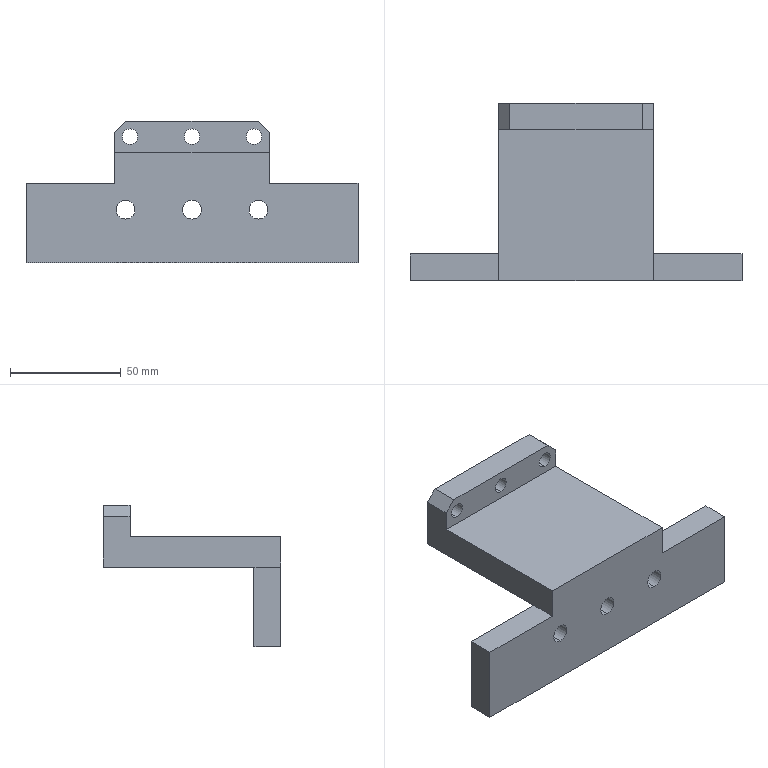NC program | NX | posted with a generic post | part box 150 x 80 x 64 mm
Lines 23 to 1152 of 10576:
(CAVITY_MILL , TOOL : D12)
N44 T09 M6
N46 G54
N48 G17 G0 G90 X82.855 Y-50.667 B0. C0. S9500 M3
N50 G43 Z30. H9
N52 Z1.004
N54 G94 G1 Z-0.496 F1000.
N56 X79.35 Y-44.597
N58 G3 X78.484 Y-44.097 R1.
N60 G1 X-78.502 F2500.
N62 G2 X-78.713 Y-44.057 R0.59
N64 X-79.056 Y-43.717 R0.765
N66 X-79.095 Y-43.519 R0.579
N68 G1 Y43.497
N70 G2 X-78.484 Y44.097 R0.624
N72 G1 X-36.84
N74 G2 X-30.496 Y47.54 R7.601
N76 G1 X30.501
N78 G2 X36.84 Y44.097 R7.601
N80 G1 X78.484
N82 G2 X79.095 Y43.497 R0.624
N84 G1 Y-43.497
N86 G2 X78.484 Y-44.097 R0.624
N88 G1 X71.895 Y-36.897
N90 X-71.895
N92 Y36.897
N94 X-38.078
N96 Y28.
N98 G3 X-30.495 Y20.46 R7.57
N100 G1 X30.495
N102 G3 X38.078 Y28. R7.57
N104 G1 Y36.897
N106 X36.638
N108 Y28.
N110 G2 X30.496 Y21.9 R6.13
N112 G1 X-30.496
N114 G2 X-36.638 Y28. R6.13
N116 G1 Y40.
N118 G2 X-30.496 Y46.1 R6.161
N120 G1 X30.496
N122 G2 X36.638 Y40. R6.161
N124 G1 Y36.897
N126 X38.078
N128 X71.895
N130 Y-36.897
N132 X64.695 Y-29.697
N134 X-64.695
N136 Y29.697
N138 X-45.278
N140 Y27.986
N142 G3 X-30.49 Y13.26 R14.77
N144 G1 X30.49
N146 G3 X45.278 Y27.986 R14.77
N148 G1 Y29.697
N150 X64.695
N152 Y-29.697
N154 X57.495 Y-22.497
N156 X-57.495
N158 Y22.497
N160 X-51.77
N162 G3 X-30.486 Y6.06 R21.97
N164 G1 X30.486
N166 G3 X51.77 Y22.497 R21.97
N168 G1 X57.495
N170 Y-22.497
N172 X50.295 Y-15.297
N174 X-50.295
N176 Y6.598
N178 G3 X-33.873 Y-0.945 R29.17
N180 G1 X-34.704 Y-8.097
N182 X-43.095
N184 Y-6.092
N186 G3 X-34.704 Y-8.097 R36.37
N188 G1 X-28.825 Y-9.297
N190 X28.825
N192 G2 X28.781 Y-7.14 R6.
N194 G1 X-28.781
N196 G2 X-28.825 Y-9.297 R6.
N198 G1 X-34.704 Y-8.097
N200 X-33.873 Y-0.945
N202 G3 X-30.483 Y-1.14 R29.17
N204 G1 X30.483
N206 G3 X50.295 Y6.598 R29.17
N208 G1 Y-15.297
N210 X43.095 Y-8.097
N212 X34.704
N214 G3 X43.095 Y-6.092 R36.37
N216 G1 Y-8.097
N218 G3 X43.595 Y-8.963 R1.
N220 G1 Z1.004
N222 G0 Z30.
N224 X82.855 Y-50.667
N226 Z0.507
N228 G1 Z-0.993 F1000.
N230 X79.35 Y-44.597
N232 G3 X78.484 Y-44.097 R1.
N234 G1 X-78.502 F2500.
N236 G2 X-78.713 Y-44.057 R0.59
N238 X-79.056 Y-43.717 R0.765
N240 X-79.095 Y-43.519 R0.579
N242 G1 Y43.497
N244 G2 X-78.484 Y44.097 R0.624
N246 G1 X-37.355
N248 G2 X-30.991 Y47.54 R7.561
N250 G1 X30.991
N252 G2 X37.355 Y44.097 R7.561
N254 G1 X78.484
N256 G2 X79.095 Y43.497 R0.624
N258 G1 Y-43.497
N260 G2 X78.484 Y-44.097 R0.624
N262 G1 X71.895 Y-36.897
N264 X-71.895
N266 Y36.897
N268 X-38.574
N270 Y28.
N272 G3 X-30.991 Y20.46 R7.569
N274 G1 X30.991
N276 G3 X38.574 Y28. R7.569
N278 G1 Y36.897
N280 X37.134
N282 Y28.
N284 G2 X30.993 Y21.9 R6.129
N286 G1 X-30.993
N288 G2 X-37.134 Y28. R6.129
N290 G1 Y40.
N292 G2 X-30.993 Y46.1 R6.121
N294 G1 X30.993
N296 G2 X37.134 Y40. R6.121
N298 G1 Y36.897
N300 X38.574
N302 X71.895
N304 Y-36.897
N306 X64.695 Y-29.697
N308 X-64.695
N310 Y29.697
N312 X-45.774
N314 Y27.986
N316 G3 X-30.986 Y13.26 R14.769
N318 G1 X30.986
N320 G3 X45.774 Y27.986 R14.769
N322 G1 Y29.697
N324 X64.695
N326 Y-29.697
N328 X57.495 Y-22.497
N330 X-57.495
N332 Y22.497
N334 X-52.266
N336 G3 X-30.982 Y6.06 R21.969
N338 G1 X30.982
N340 G3 X52.266 Y22.497 R21.969
N342 G1 X57.495
N344 Y-22.497
N346 X50.295 Y-15.297
N348 X-50.295
N350 Y6.149
N352 G3 X-34.37 Y-0.945 R29.169
N354 G1 X-35.201 Y-8.097
N356 X-43.095
N358 Y-6.272
N360 G3 X-35.201 Y-8.097 R36.369
N362 G1 X-29.322 Y-9.297
N364 X29.322
N366 G2 X29.278 Y-7.14 R6.
N368 G1 X-29.278
N370 G2 X-29.322 Y-9.297 R6.
N372 G1 X-35.201 Y-8.097
N374 X-34.37 Y-0.945
N376 G3 X-30.978 Y-1.14 R29.169
N378 G1 X30.978
N380 G3 X50.295 Y6.149 R29.169
N382 G1 Y-15.297
N384 X43.095 Y-8.097
N386 X35.201
N388 G3 X43.095 Y-6.272 R36.369
N390 G1 Y-8.097
N392 G3 X43.595 Y-8.963 R1.
N394 G1 Z0.507
N396 G0 Z30.
N398 X82.855 Y-50.667
N400 Z0.011
N402 G1 Z-1.489 F1000.
N404 X79.35 Y-44.597
N406 G3 X78.484 Y-44.097 R1.
N408 G1 X-78.502 F2500.
N410 G2 X-78.713 Y-44.057 R0.59
N412 X-79.056 Y-43.717 R0.765
N414 X-79.096 Y-43.519 R0.579
N416 G1 Y43.497
N418 G2 X-78.484 Y44.097 R0.624
N420 G1 X-37.862
N422 G2 X-32.26 Y47.476 R7.489
N424 G1 X-31.62 Y47.534
N426 X-31.489 Y47.54
N428 X31.496
N430 G2 X37.632 Y44.422 R7.67
N432 X37.858 Y44.097 R7.373
N434 G1 X78.484
N436 G2 X79.096 Y43.497 R0.624
N438 G1 Y-43.497
N440 G2 X78.484 Y-44.097 R0.624
N442 G1 X71.896 Y-36.897
N444 X-71.896
N446 Y36.897
N448 X-39.071
N450 Y28.
N452 G3 X-31.488 Y20.46 R7.575
N454 G1 X31.489
N456 G3 X39.071 Y28. R7.575
N458 G1 Y36.897
N460 X37.631
N462 Y28.
N464 G2 X31.489 Y21.9 R6.135
N466 G1 X-31.489
N468 G2 X-37.631 Y28. R6.135
N470 G1 Y40.017
N472 G2 X-32.13 Y46.042 R6.049
N474 G1 X-31.489 Y46.1
N476 X31.489
N478 G2 X36.473 Y43.567 R6.23
N480 X37.631 Y40.046 R5.933
N482 G1 Y36.897
N484 X39.071
N486 X71.896
N488 Y-36.897
N490 X64.696 Y-29.697
N492 X-64.696
N494 Y29.697
N496 X-46.271
N498 Y27.983
N500 G3 X-31.484 Y13.26 R14.775
N502 G1 X31.487
N504 G3 X46.271 Y27.983 R14.775
N506 G1 Y29.697
N508 X64.696
N510 Y-29.697
N512 X57.496 Y-22.497
N514 X-57.496
N516 Y22.497
N518 X-52.762
N520 G3 X-31.482 Y6.06 R21.975
N522 G1 X31.484
N524 G3 X52.762 Y22.497 R21.975
N526 G1 X57.496
N528 Y-22.497
N530 X50.296 Y-15.297
N532 X-50.296
N534 Y5.724
N536 G3 X-34.862 Y-0.945 R29.175
N538 G1 X-35.692 Y-8.097
N540 X-43.096
N542 Y-6.441
N544 G3 X-35.692 Y-8.097 R36.375
N546 G1 X-29.813 Y-9.297
N548 X29.813
N550 G2 X29.769 Y-7.14 R6.
N552 G1 X-29.769
N554 G2 X-29.813 Y-9.297 R6.
N556 G1 X-35.692 Y-8.097
N558 X-34.862 Y-0.945
N560 G3 X-31.479 Y-1.14 R29.175
N562 G1 X31.482
N564 G3 X50.296 Y5.724 R29.175
N566 G1 Y-15.297
N568 X43.096 Y-8.097
N570 X35.692
N572 G3 X43.096 Y-6.441 R36.375
N574 G1 Y-8.097
N576 G3 X43.596 Y-8.963 R1.
N578 G1 Z0.011
N580 G0 X82.854 Y-50.667 Z-0.486
N582 G1 Z-1.986 F1000.
N584 X79.35 Y-44.597
N586 G3 X78.484 Y-44.097 R1.
N588 G1 X-78.502 F2500.
N590 G2 X-78.713 Y-44.057 R0.59
N592 X-79.056 Y-43.717 R0.765
N594 X-79.096 Y-43.519 R0.579
N596 G1 Y43.497
N598 G2 X-78.484 Y44.097 R0.624
N600 G1 X-38.336
N602 G2 X-31.986 Y47.54 R7.585
N604 G1 X31.987
N606 G2 X38.336 Y44.097 R7.585
N608 G1 X78.484
N610 G2 X79.096 Y43.497 R0.624
N612 G1 Y-43.497
N614 G2 X78.484 Y-44.097 R0.624
N616 G1 X71.896 Y-36.897
N618 X-71.896
N620 Y36.897
N622 X-39.567
N624 Y28.
N626 G3 X-31.983 Y20.46 R7.561
N628 G1 X31.983
N630 G3 X39.567 Y28. R7.561
N632 G1 Y36.897
N634 X38.127
N636 Y28.
N638 G2 X31.986 Y21.9 R6.121
N640 G1 X-31.986
N642 G2 X-38.127 Y28. R6.121
N644 G1 Y40.
N646 G2 X-31.986 Y46.1 R6.145
N648 G1 X31.986
N650 G2 X38.127 Y40. R6.145
N652 G1 Y36.897
N654 X39.567
N656 X71.896
N658 Y-36.897
N660 X64.696 Y-29.697
N662 X-64.696
N664 Y29.697
N666 X-46.767
N668 Y27.99
N670 G3 X-31.974 Y13.26 R14.761
N672 G1 X31.974
N674 G3 X46.767 Y27.99 R14.761
N676 G1 Y29.697
N678 X64.696
N680 Y-29.697
N682 X57.496 Y-22.497
N684 X-57.496
N686 Y22.497
N688 X-53.261
N690 G3 X-31.967 Y6.06 R21.961
N692 G1 X31.967
N694 G3 X53.261 Y22.497 R21.961
N696 G1 X57.496
N698 Y-22.497
N700 X50.296 Y-15.297
N702 X-50.296
N704 Y5.308
N706 G3 X-35.371 Y-0.945 R29.161
N708 G1 X-36.202 Y-8.097
N710 X-43.096
N712 Y-6.608
N714 G3 X-36.202 Y-8.097 R36.361
N716 G1 X-30.323 Y-9.297
N718 X30.323
N720 G2 X30.279 Y-7.14 R6.
N722 G1 X-30.279
N724 G2 X-30.323 Y-9.297 R6.
N726 G1 X-36.202 Y-8.097
N728 X-35.371 Y-0.945
N730 G3 X-31.961 Y-1.14 R29.161
N732 G1 X31.961
N734 G3 X50.296 Y5.308 R29.161
N736 G1 Y-15.297
N738 X43.096 Y-8.097
N740 X36.202
N742 G3 X43.096 Y-6.608 R36.361
N744 G1 Y-8.097
N746 G3 X43.596 Y-8.963 R1.
N748 G1 Z-0.486
N750 G0 X82.854 Y-50.667 Z-0.982
N752 G1 Z-2.482 F1000.
N754 X79.35 Y-44.597
N756 G3 X78.484 Y-44.097 R1.
N758 G1 X-78.502 F2500.
N760 G2 X-78.713 Y-44.057 R0.59
N762 X-79.056 Y-43.717 R0.766
N764 X-79.096 Y-43.519 R0.58
N766 G1 Y43.497
N768 G2 X-78.484 Y44.097 R0.624
N770 G1 X-38.839
N772 G2 X-32.482 Y47.54 R7.571
N774 G1 X32.481
N776 G2 X38.839 Y44.097 R7.571
N778 G1 X78.484
N780 G2 X79.096 Y43.497 R0.624
N782 G1 Y-43.497
N784 G2 X78.484 Y-44.097 R0.624
N786 G1 X71.896 Y-36.897
N788 X-71.896
N790 Y36.897
N792 X-40.064
N794 Y28.
N796 G3 X-32.48 Y20.46 R7.567
N798 G1 X32.48
N800 G3 X40.064 Y28. R7.567
N802 G1 Y36.897
N804 X38.624
N806 Y28.
N808 G2 X32.482 Y21.9 R6.127
N810 G1 X-32.482
N812 G2 X-38.624 Y28. R6.127
N814 G1 Y40.
N816 G2 X-32.482 Y46.1 R6.131
N818 G1 X32.482
N820 G2 X38.624 Y40. R6.131
N822 G1 Y36.897
N824 X40.064
N826 X71.896
N828 Y-36.897
N830 X64.696 Y-29.697
N832 X-64.696
N834 Y29.697
N836 X-47.264
N838 Y27.987
N840 G3 X-32.474 Y13.26 R14.767
N842 G1 X32.474
N844 G3 X47.264 Y27.987 R14.767
N846 G1 Y29.697
N848 X64.696
N850 Y-29.697
N852 X57.496 Y-22.497
N854 X-57.496
N856 Y22.497
N858 X-53.756
N860 G3 X-32.469 Y6.06 R21.967
N862 G1 X32.469
N864 G3 X53.756 Y22.497 R21.967
N866 G1 X57.496
N868 Y-22.497
N870 X50.296 Y-15.297
N872 X-50.296
N874 Y4.921
N876 G3 X-35.861 Y-0.945 R29.167
N878 G1 X-36.692 Y-8.097
N880 X-43.096
N882 Y-6.761
N884 G3 X-36.692 Y-8.097 R36.367
N886 G1 X-30.813 Y-9.297
N888 X30.813
N890 G2 X30.769 Y-7.14 R6.
N892 G1 X-30.769
N894 G2 X-30.813 Y-9.297 R6.
N896 G1 X-36.692 Y-8.097
N898 X-35.861 Y-0.945
N900 G3 X-32.465 Y-1.14 R29.167
N902 G1 X32.465
N904 G3 X50.296 Y4.921 R29.167
N906 G1 Y-15.297
N908 X43.096 Y-8.097
N910 X36.692
N912 G3 X43.096 Y-6.761 R36.367
N914 G1 Y-8.097
N916 G3 X43.596 Y-8.963 R1.
N918 G1 Z-0.982
N920 G0 X82.854 Y-50.667 Z-1.479
N922 G1 Z-2.979 F1000.
N924 X79.35 Y-44.597
N926 G3 X78.484 Y-44.097 R1.
N928 G1 X-78.502 F2500.
N930 G2 X-78.713 Y-44.057 R0.59
N932 X-79.056 Y-43.717 R0.766
N934 X-79.096 Y-43.519 R0.58
N936 G1 Y43.497
N938 G2 X-78.484 Y44.097 R0.625
N940 G1 X-39.33
N942 G2 X-32.979 Y47.54 R7.583
N944 G1 X32.979
N946 G2 X39.33 Y44.097 R7.583
N948 G1 X78.484
N950 G2 X79.096 Y43.497 R0.625
N952 G1 Y-43.497
N954 G2 X78.484 Y-44.097 R0.625
N956 G1 X71.896 Y-36.897
N958 X-71.896
N960 Y36.897
N962 X-40.56
N964 Y28.
N966 G3 X-32.977 Y20.46 R7.565
N968 G1 X32.977
N970 G3 X40.56 Y28. R7.565
N972 G1 Y36.897
N974 X39.12
N976 Y28.
N978 G2 X32.979 Y21.9 R6.125
N980 G1 X-32.979
N982 G2 X-39.12 Y28. R6.125
N984 G1 Y40.
N986 G2 X-32.979 Y46.1 R6.143
N988 G1 X32.979
N990 G2 X39.12 Y40. R6.143
N992 G1 Y36.897
N994 X40.56
N996 X71.896
N998 Y-36.897
N1000 X64.696 Y-29.697
N1002 X-64.696
N1004 Y29.697
N1006 X-47.76
N1008 Y27.988
N1010 G3 X-32.969 Y13.26 R14.765
N1012 G1 X32.969
N1014 G3 X47.76 Y27.988 R14.765
N1016 G1 Y29.697
N1018 X64.696
N1020 Y-29.697
N1022 X57.496 Y-22.497
N1024 X-57.496
N1026 Y22.497
N1028 X-54.253
N1030 G3 X-32.964 Y6.06 R21.965
N1032 G1 X32.964
N1034 G3 X54.253 Y22.497 R21.965
N1036 G1 X57.496
N1038 Y-22.497
N1040 X50.296 Y-15.297
N1042 X-50.296
N1044 Y4.545
N1046 G3 X-36.36 Y-0.945 R29.165
N1048 G1 X-37.19 Y-8.097
N1050 X-43.096
N1052 Y-6.909
N1054 G3 X-37.19 Y-8.097 R36.365
N1056 G1 X-31.311 Y-9.297
N1058 X31.311
N1060 G2 X31.267 Y-7.14 R6.
N1062 G1 X-31.267
N1064 G2 X-31.311 Y-9.297 R6.
N1066 G1 X-37.19 Y-8.097
N1068 X-36.36 Y-0.945
N1070 G3 X-32.959 Y-1.14 R29.165
N1072 G1 X32.959
N1074 G3 X50.296 Y4.545 R29.165
N1076 G1 Y-15.297
N1078 X43.096 Y-8.097
N1080 X37.19
N1082 G3 X43.096 Y-6.909 R36.365
N1084 G1 Y-8.097
N1086 G3 X43.596 Y-8.963 R1.
N1088 G1 Z-1.479
N1090 G0 X82.854 Y-50.667 Z-1.975
N1092 G1 Z-3.475 F1000.
N1094 X79.35 Y-44.597
N1096 G3 X78.484 Y-44.097 R1.
N1098 G1 X-78.502 F2500.
N1100 G2 X-78.713 Y-44.057 R0.59
N1102 X-79.056 Y-43.717 R0.766
N1104 X-79.096 Y-43.519 R0.58
N1106 G1 Y43.497
N1108 G2 X-78.484 Y44.097 R0.625
N1110 G1 X-39.837
N1112 G2 X-33.473 Y47.54 R7.561
N1114 G1 X33.473
N1116 G2 X39.837 Y44.097 R7.561
N1118 G1 X78.484
N1120 G2 X79.096 Y43.497 R0.625
N1122 G1 Y-43.497
N1124 G2 X78.484 Y-44.097 R0.625
N1126 G1 X71.896 Y-36.897
N1128 X-71.896
N1130 Y36.897
N1132 X-41.056
N1134 Y28.
N1136 G3 X-33.474 Y20.46 R7.57
N1138 G1 X33.474
N1140 G3 X41.056 Y28. R7.57
N1142 G1 Y36.897
N1144 X39.616
N1146 Y28.
N1148 G2 X33.475 Y21.9 R6.13
N1150 G1 X-33.475
N1152 G2 X-39.616 Y28. R6.13
N1154 G1 Y40.
N1156 G2 X-33.475 Y46.1 R6.121
N1158 G1 X33.475
N1160 G2 X39.616 Y40. R6.121
N1162 G1 Y36.897
N1164 X41.056
N1166 X71.896
N1168 Y-36.897
N1170 X64.696 Y-29.697
N1172 X-64.696
N1174 Y29.697
N1176 X-48.256
N1178 Y27.985
N1180 G3 X-33.469 Y13.26 R14.77
N1182 G1 X33.469
N1184 G3 X48.256 Y27.985 R14.77
N1186 G1 Y29.697
N1188 X64.696
N1190 Y-29.697
N1192 X57.496 Y-22.497
N1194 X-57.496
N1196 Y22.497
N1198 X-54.748
N1200 G3 X-33.465 Y6.06 R21.97
N1202 G1 X33.465
N1204 G3 X54.748 Y22.497 R21.97
N1206 G1 X57.496
N1208 Y-22.497
N1210 X50.296 Y-15.297
N1212 X-50.296
N1214 Y4.19
N1216 G3 X-36.851 Y-0.945 R29.17
N1218 G1 X-37.681 Y-8.097
N1220 X-43.096
N1222 Y-7.048
N1224 G3 X-37.681 Y-8.097 R36.37
N1226 G1 X-31.802 Y-9.297
N1228 X31.802
N1230 G2 X31.758 Y-7.14 R6.
N1232 G1 X-31.758
N1234 G2 X-31.802 Y-9.297 R6.
N1236 G1 X-37.681 Y-8.097
N1238 X-36.851 Y-0.945
N1240 G3 X-33.462 Y-1.14 R29.17
N1242 G1 X33.462
N1244 G3 X50.296 Y4.19 R29.17
N1246 G1 Y-15.297
N1248 X43.096 Y-8.097
N1250 X37.681
N1252 G3 X43.096 Y-7.048 R36.37
N1254 G1 Y-8.097
N1256 G3 X43.596 Y-8.963 R1.
N1258 G1 Z-1.975
N1260 G0 X82.854 Y-50.668 Z-2.471
N1262 G1 Z-3.971 F1000.
N1264 X79.35 Y-44.597
N1266 G3 X78.484 Y-44.097 R1.
N1268 G1 X-78.502 F2500.
N1270 G2 X-78.713 Y-44.057 R0.59
N1272 X-79.056 Y-43.717 R0.766
N1274 X-79.096 Y-43.519 R0.58
N1276 G1 Y43.497
N1278 G2 X-78.484 Y44.097 R0.625
N1280 G1 X-40.323
N1282 G2 X-33.971 Y47.54 R7.583
N1284 G1 X33.972
N1286 G2 X40.323 Y44.097 R7.583
N1288 G1 X78.484
N1290 G2 X79.096 Y43.497 R0.625
N1292 G1 Y-43.497
N1294 G2 X78.484 Y-44.097 R0.625
N1296 G1 X71.896 Y-36.897
N1298 X-71.896
N1300 Y36.897
N1302 X-41.553
N1304 Y27.992
N1306 G3 X-33.97 Y20.46 R7.575
N1308 G1 X33.971
N1310 G3 X41.553 Y28. R7.575
N1312 G1 Y36.897
N1314 X40.113
N1316 Y28.
N1318 G2 X33.971 Y21.9 R6.135
N1320 G1 X-33.971
N1322 G2 X-40.113 Y28. R6.135
N1324 G1 Y40.
N1326 G2 X-33.971 Y46.1 R6.143
N1328 G1 X33.971
N1330 G2 X40.113 Y40. R6.143
N1332 G1 Y36.897
N1334 X41.553
N1336 X71.896
N1338 Y-36.897
N1340 X64.696 Y-29.697
N1342 X-64.696
N1344 Y29.697
N1346 X-48.753
N1348 Y27.971
N1350 G3 X-33.967 Y13.26 R14.775
N1352 G1 X33.969
N1354 G3 X48.753 Y27.983 R14.775
N1356 G1 Y29.697
N1358 X64.696
N1360 Y-29.697
N1362 X57.496 Y-22.497
N1364 X-57.496
N1366 Y22.497
N1368 X-55.244
N1370 G3 X-33.964 Y6.06 R21.975
N1372 G1 X33.967
N1374 G3 X55.244 Y22.497 R21.975
N1376 G1 X57.496
N1378 Y-22.497
N1380 X50.296 Y-15.297
N1382 X-50.296
N1384 Y3.85
N1386 G3 X-37.343 Y-0.945 R29.175
N1388 G1 X-38.173 Y-8.097
N1390 X-43.096
N1392 Y-7.179
N1394 G3 X-38.173 Y-8.097 R36.375
N1396 G1 X-32.294 Y-9.297
N1398 X32.294
N1400 G2 X32.25 Y-7.14 R6.
N1402 G1 X-32.25
N1404 G2 X-32.294 Y-9.297 R6.
N1406 G1 X-38.173 Y-8.097
N1408 X-37.343 Y-0.945
N1410 G3 X-33.962 Y-1.14 R29.175
N1412 G1 X33.965
N1414 G3 X50.296 Y3.85 R29.175
N1416 G1 Y-15.297
N1418 X43.096 Y-8.097
N1420 X38.173
N1422 G3 X43.096 Y-7.179 R36.375
N1424 G1 Y-8.097
N1426 G3 X43.596 Y-8.963 R1.
N1428 G1 Z-2.471
N1430 G0 X82.854 Y-50.668 Z-2.968
N1432 G1 Z-4.468 F1000.
N1434 X79.35 Y-44.597
N1436 G3 X78.484 Y-44.097 R1.
N1438 G1 X-78.502 F2500.
N1440 G2 X-78.713 Y-44.057 R0.59
N1442 X-79.056 Y-43.717 R0.767
N1444 X-79.096 Y-43.519 R0.58
N1446 G1 Y43.497
N1448 G2 X-78.484 Y44.097 R0.625
N1450 G1 X-40.814
N1452 G2 X-34.468 Y47.54 R7.595
N1454 G1 X34.471
N1456 G2 X40.814 Y44.097 R7.595
N1458 G1 X78.484
N1460 G2 X79.096 Y43.497 R0.625
N1462 G1 Y-43.497
N1464 G2 X78.484 Y-44.097 R0.625
N1466 G1 X71.896 Y-36.897
N1468 X-71.896
N1470 Y36.897
N1472 X-42.049
N1474 Y28.
N1476 G3 X-34.466 Y20.46 R7.565
N1478 G1 X34.502
N1480 X34.673 Y20.464
N1482 X34.78 Y20.471
N1484 X35.273 Y20.519
N1486 G3 X42.049 Y27.991 R7.507
N1488 G1 Y36.897
N1490 X40.609
N1492 Y27.991
N1494 G2 X35.133 Y21.952 R6.067
N1496 G1 X34.639 Y21.904
N1498 X34.468 Y21.9
N1500 X-34.468
N1502 G2 X-40.609 Y28. R6.125
N1504 G1 Y40.
N1506 G2 X-34.468 Y46.1 R6.155
N1508 G1 X34.468
N1510 G2 X40.609 Y40. R6.155
N1512 G1 Y36.897
N1514 X42.049
N1516 X71.896
N1518 Y-36.897
N1520 X64.696 Y-29.697
N1522 X-64.696
N1524 Y29.697
N1526 X-49.249
N1528 Y27.988
N1530 G3 X-34.459 Y13.26 R14.765
N1532 G1 X34.51
N1534 X34.629 Y13.261
N1536 X34.843 Y13.266
N1538 G3 X35.481 Y13.305 R8.64
N1540 G1 X35.974 Y13.353
N1542 G3 X49.249 Y27.991 R14.707
N1544 G1 Y29.697
N1546 X64.696
N1548 Y-29.697
N1550 X57.496 Y-22.497
N1552 X-57.496
N1554 Y22.497
N1556 X-55.742
N1558 G3 X-34.453 Y6.06 R21.965
N1560 G1 X34.553
N1562 X34.756 Y6.062
N1564 X35.013 Y6.068
N1566 G3 X36.182 Y6.139 R15.84
N1568 X55.749 Y22.497 R21.907
N1570 G1 X57.496
N1572 Y-22.497
N1574 X50.296 Y-15.297
N1576 X-50.296
N1578 Y3.518
N1580 G3 X-37.848 Y-0.945 R29.165
N1582 G1 X-38.679 Y-8.097
N1584 X-43.096
N1586 Y-7.306
N1588 G3 X-38.679 Y-8.097 R36.365
N1590 G1 X-32.8 Y-9.297
N1592 X32.697
N1594 G2 X32.653 Y-7.14 R6.
N1596 G1 X-32.756
N1598 G2 X-32.8 Y-9.297 R6.
N1600 G1 X-38.679 Y-8.097
N1602 X-37.848 Y-0.945
N1604 G3 X-34.448 Y-1.14 R29.165
N1606 G1 X34.595
N1608 X34.884 Y-1.137
N1610 X35.182 Y-1.13
N1612 G3 X36.801 Y-1.034 R23.04
N1614 X50.296 Y3.51 R29.107
N1616 G1 Y-15.297
N1618 X43.096 Y-8.097
N1620 X38.576
N1622 G3 X43.096 Y-7.3 R36.307
N1624 G1 Y-8.097
N1626 G3 X43.596 Y-8.963 R1.
N1628 G1 Z-2.968
N1630 G0 X82.854 Y-50.668 Z-3.464
N1632 G1 Z-4.964 F1000.
N1634 X79.35 Y-44.597
N1636 G3 X78.484 Y-44.097 R1.
N1638 G1 X-78.502 F2500.
N1640 G2 X-78.713 Y-44.057 R0.59
N1642 X-79.056 Y-43.717 R0.767
N1644 X-79.096 Y-43.519 R0.58
N1646 G1 Y43.497
N1648 G2 X-78.484 Y44.097 R0.625
N1650 G1 X-41.316
N1652 G2 X-34.963 Y47.54 R7.555
N1654 G1 X34.963
N1656 G2 X41.316 Y44.097 R7.555
N1658 G1 X78.484
N1660 G2 X79.096 Y43.497 R0.625
N1662 G1 Y-43.497
N1664 G2 X78.484 Y-44.097 R0.625
N1666 G1 X71.896 Y-36.897
N1668 X-71.896
N1670 Y36.897
N1672 X-42.533
N1674 Y28.
N1676 G3 X-34.963 Y20.46 R7.555
N1678 G1 X34.963
N1680 G3 X42.533 Y28. R7.555
N1682 G1 Y36.897
N1684 X41.093
N1686 Y28.
N1688 G2 X34.964 Y21.9 R6.115
N1690 G1 X-34.964
N1692 G2 X-41.093 Y28. R6.115
N1694 G1 Y40.
N1696 G2 X-34.964 Y46.1 R6.115
N1698 G1 X34.964
N1700 G2 X41.093 Y40. R6.115
N1702 G1 Y36.897
N1704 X42.533
N1706 X71.896
N1708 Y-36.897
N1710 X64.696 Y-29.697
N1712 X-64.696
N1714 Y29.697
N1716 X-49.733
N1718 Y27.993
N1720 G3 X-34.956 Y13.26 R14.755
N1722 G1 X34.956
N1724 G3 X49.733 Y27.993 R14.755
N1726 G1 Y29.697
N1728 X64.696
N1730 Y-29.697
N1732 X57.496 Y-22.497
N1734 X-57.496
N1736 Y22.497
N1738 X-56.229
N1740 G3 X-34.951 Y6.06 R21.955
N1742 G1 X34.951
N1744 G3 X56.229 Y22.497 R21.955
N1746 G1 X57.496
N1748 Y-22.497
N1750 X50.296 Y-15.297
N1752 X-50.296
N1754 Y3.208
N1756 G3 X-38.342 Y-0.945 R29.155
N1758 G1 X-39.172 Y-8.097
N1760 X-43.096
N1762 Y-7.422
N1764 G3 X-39.172 Y-8.097 R36.355
N1766 G1 X-33.294 Y-9.297
N1768 X33.294
N1770 G2 X33.249 Y-7.14 R6.
N1772 G1 X-33.249
N1774 G2 X-33.294 Y-9.297 R6.
N1776 G1 X-39.172 Y-8.097
N1778 X-38.342 Y-0.945
N1780 G3 X-34.947 Y-1.14 R29.155
N1782 G1 X34.947
N1784 G3 X50.296 Y3.208 R29.155
N1786 G1 Y-15.297
N1788 X43.096 Y-8.097
N1790 X39.172
N1792 G3 X43.096 Y-7.422 R36.355
N1794 G1 Y-8.097
N1796 G3 X43.596 Y-8.963 R1.
N1798 G1 Z-3.464
N1800 G0 X82.854 Y-50.668 Z-3.961
N1802 G1 Z-5.461 F1000.
N1804 X79.35 Y-44.597
N1806 G3 X78.484 Y-44.097 R1.
N1808 G1 X-78.502 F2500.
N1810 G2 X-78.713 Y-44.057 R0.59
N1812 X-79.056 Y-43.717 R0.767
N1814 X-79.096 Y-43.519 R0.58
N1816 G1 Y43.497
N1818 G2 X-78.484 Y44.097 R0.625
N1820 G1 X-41.33
N1822 G2 X-35. Y47.54 R7.54
N1824 G1 X35.
N1826 G2 X41.33 Y44.097 R7.54
N1828 G1 X78.484
N1830 G2 X79.096 Y43.497 R0.625
N1832 G1 Y-43.497
N1834 G2 X78.484 Y-44.097 R0.625
N1836 G1 X71.896 Y-36.897
N1838 X-71.896
N1840 Y36.897
N1842 X-42.54
N1844 Y28.
N1846 G3 X-35. Y20.46 R7.54
N1848 G1 X35.
N1850 G3 X42.54 Y28. R7.54
N1852 G1 Y36.897
N1854 X41.1
N1856 Y28.
N1858 G2 X35. Y21.9 R6.1
N1860 G1 X-35.
N1862 G2 X-41.1 Y28. R6.1
N1864 G1 Y40.
N1866 G2 X-35. Y46.1 R6.1
N1868 G1 X35.
N1870 G2 X41.1 Y40. R6.1
N1872 G1 Y36.897
N1874 X42.54
N1876 X71.896
N1878 Y-36.897
N1880 X64.696 Y-29.697
N1882 X-64.696
N1884 Y29.697
N1886 X-49.74
N1888 Y28.
N1890 G3 X-35. Y13.26 R14.74
N1892 G1 X35.
N1894 G3 X49.74 Y28. R14.74
N1896 G1 Y29.697
N1898 X64.696
N1900 Y-29.697
N1902 X57.496 Y-22.497
N1904 X-57.496
N1906 Y22.497
N1908 X-56.239
N1910 G3 X-35. Y6.06 R21.94
N1912 G1 X35.
N1914 G3 X56.239 Y22.497 R21.94
N1916 G1 X57.496
N1918 Y-22.497
N1920 X50.296 Y-15.297
N1922 X-50.296
N1924 Y3.197
N1926 G3 X-38.362 Y-0.945 R29.14
N1928 G1 X-39.192 Y-8.097
N1930 X-43.096
N1932 Y-7.427
N1934 G3 X-39.192 Y-8.097 R36.34
N1936 G1 X-33.314 Y-9.297
N1938 X33.314
N1940 G2 X33.269 Y-7.14 R6.
N1942 G1 X-33.269
N1944 G2 X-33.314 Y-9.297 R6.
N1946 G1 X-39.192 Y-8.097
N1948 X-38.362 Y-0.945
N1950 G3 X-35. Y-1.14 R29.14
N1952 G1 X35.
N1954 G3 X50.296 Y3.197 R29.14
N1956 G1 Y-15.297
N1958 X43.096 Y-8.097
N1960 X39.192
N1962 G3 X43.096 Y-7.427 R36.34
N1964 G1 Y-8.097
N1966 G3 X43.596 Y-8.963 R1.
N1968 G1 Z-3.961
N1970 G0 X82.854 Y-50.668 Z-4.457
N1972 G1 Z-5.957 F1000.
N1974 X79.35 Y-44.597
N1976 G3 X78.484 Y-44.097 R1.
N1978 G1 X-78.502 F2500.
N1980 G2 X-78.713 Y-44.057 R0.59
N1982 X-79.056 Y-43.717 R0.767
N1984 X-79.096 Y-43.519 R0.581
N1986 G1 Y43.497
N1988 G2 X-78.484 Y44.097 R0.625
N1990 G1 X-41.33
N1992 G2 X-35. Y47.54 R7.54
N1994 G1 X35.
N1996 G2 X41.33 Y44.097 R7.54
N1998 G1 X78.484
N2000 G2 X79.096 Y43.497 R0.625
N2002 G1 Y-43.497
N2004 G2 X78.484 Y-44.097 R0.625
N2006 G1 X71.896 Y-36.897
N2008 X-71.896
N2010 Y36.897
N2012 X-42.54
N2014 Y28.
N2016 G3 X-35. Y20.46 R7.54
N2018 G1 X35.
N2020 G3 X42.54 Y28. R7.54
N2022 G1 Y36.897
N2024 X41.1
N2026 Y28.
N2028 G2 X35. Y21.9 R6.1
N2030 G1 X-35.
N2032 G2 X-41.1 Y28. R6.1
N2034 G1 Y40.
N2036 G2 X-35. Y46.1 R6.1
N2038 G1 X35.
N2040 G2 X41.1 Y40. R6.1
N2042 G1 Y36.897
N2044 X42.54
N2046 X71.896
N2048 Y-36.897
N2050 X64.696 Y-29.697
N2052 X-64.696
N2054 Y29.697
N2056 X-49.74
N2058 Y28.
N2060 G3 X-35. Y13.26 R14.74
N2062 G1 X35.
N2064 G3 X49.74 Y28. R14.74
N2066 G1 Y29.697
N2068 X64.696
N2070 Y-29.697
N2072 X57.496 Y-22.497
N2074 X-57.496
N2076 Y22.497
N2078 X-56.239
N2080 G3 X-35. Y6.06 R21.94
N2082 G1 X35.
N2084 G3 X56.239 Y22.497 R21.94
N2086 G1 X57.496
N2088 Y-22.497
N2090 X50.296 Y-15.297
N2092 X-50.296
N2094 Y3.197
N2096 G3 X-38.362 Y-0.945 R29.14
N2098 G1 X-39.192 Y-8.097
N2100 X-43.096
N2102 Y-7.427
N2104 G3 X-39.192 Y-8.097 R36.34
N2106 G1 X-33.313 Y-9.297
N2108 X33.313
N2110 G2 X33.269 Y-7.14 R6.
N2112 G1 X-33.269
N2114 G2 X-33.313 Y-9.297 R6.
N2116 G1 X-39.192 Y-8.097
N2118 X-38.362 Y-0.945
N2120 G3 X-35. Y-1.14 R29.14
N2122 G1 X35.
N2124 G3 X50.296 Y3.197 R29.14
N2126 G1 Y-15.297
N2128 X43.096 Y-8.097
N2130 X39.192
N2132 G3 X43.096 Y-7.427 R36.34
N2134 G1 Y-8.097
N2136 G3 X43.596 Y-8.963 R1.
N2138 G1 Z-4.457
N2140 G0 X82.854 Y-50.668 Z-4.954
N2142 G1 Z-6.454 F1000.
N2144 X79.35 Y-44.597
N2146 G3 X78.484 Y-44.097 R1.
N2148 G1 X-78.502 F2500.
N2150 G2 X-78.713 Y-44.057 R0.59
N2152 X-79.056 Y-43.716 R0.768
N2154 X-79.096 Y-43.519 R0.581
N2156 G1 Y43.497
N2158 G2 X-78.484 Y44.097 R0.625
N2160 G1 X-41.33
N2162 G2 X-35. Y47.54 R7.54
N2164 G1 X35.
N2166 G2 X41.33 Y44.097 R7.54
N2168 G1 X78.484
N2170 G2 X79.096 Y43.497 R0.625
N2172 G1 Y-43.497
N2174 G2 X78.484 Y-44.097 R0.625
N2176 G1 X71.896 Y-36.897
N2178 X-71.896
N2180 Y36.897
N2182 X-42.54
N2184 Y28.
N2186 G3 X-35. Y20.46 R7.54
N2188 G1 X35.
N2190 G3 X42.54 Y28. R7.54
N2192 G1 Y36.897
N2194 X41.1
N2196 Y28.
N2198 G2 X35. Y21.9 R6.1
N2200 G1 X-35.
N2202 G2 X-41.1 Y28. R6.1
N2204 G1 Y40.
N2206 G2 X-35. Y46.1 R6.1
N2208 G1 X35.
N2210 G2 X41.1 Y40. R6.1
N2212 G1 Y36.897
N2214 X42.54
N2216 X71.896
N2218 Y-36.897
N2220 X64.696 Y-29.697
N2222 X-64.696
N2224 Y29.697
N2226 X-49.74
N2228 Y28.
N2230 G3 X-35. Y13.26 R14.74
N2232 G1 X35.
N2234 G3 X49.74 Y28. R14.74
N2236 G1 Y29.697
N2238 X64.696
N2240 Y-29.697
N2242 X57.496 Y-22.497
N2244 X-57.496
N2246 Y22.497
N2248 X-56.239
N2250 G3 X-35. Y6.06 R21.94
N2252 G1 X35.
N2254 G3 X56.239 Y22.497 R21.94
N2256 G1 X57.496
N2258 Y-22.497
N2260 X50.296 Y-15.297
N2262 X-50.296
N2264 Y3.197
N2266 G3 X-38.361 Y-0.945 R29.14
N2268 G1 X-39.192 Y-8.097
N2270 X-43.096
N2272 Y-7.427
N2274 G3 X-39.192 Y-8.097 R36.34
N2276 G1 X-33.313 Y-9.297
N2278 X33.313
N2280 G2 X33.269 Y-7.14 R6.
N2282 G1 X-33.269
N2284 G2 X-33.313 Y-9.297 R6.
N2286 G1 X-39.192 Y-8.097
N2288 X-38.361 Y-0.945
N2290 G3 X-35. Y-1.14 R29.14
N2292 G1 X35.
N2294 G3 X50.296 Y3.197 R29.14
N2296 G1 Y-15.297